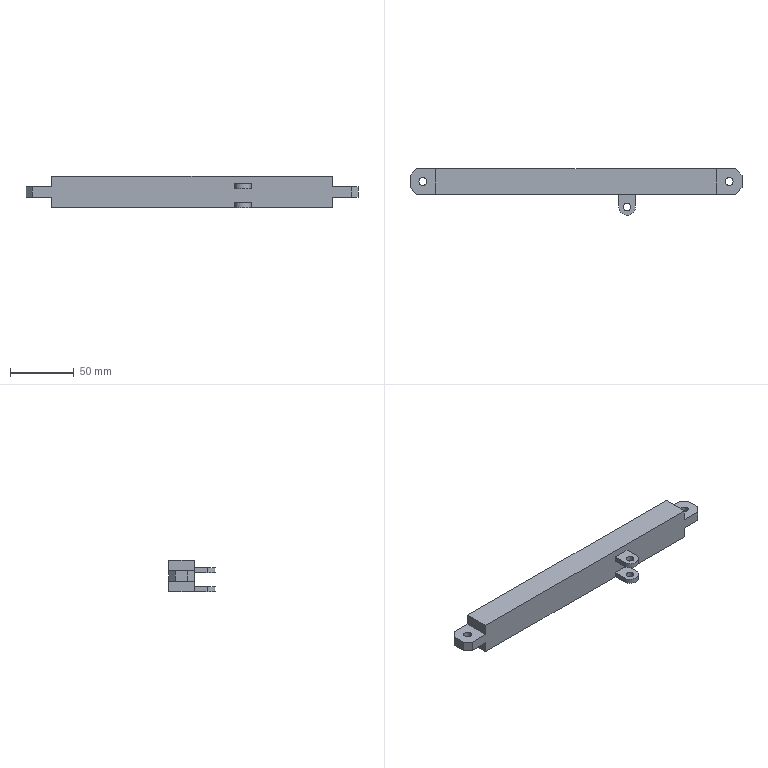Part | SolidWorks | features ICE 3, Chamfer 1, Extrusion 1, LPattern 1, MirrorPattern 1 | 1 solid | 35 faces | box 260 x 36.5 x 25 mm | volume 116892 mm3 | plane 25 | cylinder 10 | commonest cylinder face diameters 6 x8 13 x2
STEP:
#1=CARTESIAN_POINT('',(43.,-20.,6.5));
#2=VERTEX_POINT('',#1);
#3=CARTESIAN_POINT('',(37.,-20.,6.5));
#4=VERTEX_POINT('',#3);
#5=CARTESIAN_POINT('',(40.,-20.,6.5));
#6=DIRECTION('',(0.,0.,-1.));
#7=DIRECTION('',(-1.,0.,0.));
#8=AXIS2_PLACEMENT_3D('',#5,#6,#7);
#9=CIRCLE('',#8,3.);
#10=EDGE_CURVE('',#2,#4,#9,.T.);
#11=ORIENTED_EDGE('',*,*,#10,.F.);
#12=CARTESIAN_POINT('',(43.,-20.,2.5));
#13=VERTEX_POINT('',#12);
#14=CARTESIAN_POINT('',(43.,-20.,6.5));
#15=DIRECTION('',(0.,0.,-1.));
#16=VECTOR('',#15,1000.);
#17=LINE('',#14,#16);
#18=EDGE_CURVE('',#2,#13,#17,.T.);
#19=ORIENTED_EDGE('',*,*,#18,.T.);
#20=CARTESIAN_POINT('',(37.,-20.,2.5));
#21=VERTEX_POINT('',#20);
#22=CARTESIAN_POINT('',(40.,-20.,2.5));
#23=DIRECTION('',(0.,0.,-1.));
#24=DIRECTION('',(-1.,0.,0.));
#25=AXIS2_PLACEMENT_3D('',#22,#23,#24);
#26=CIRCLE('',#25,3.);
#27=EDGE_CURVE('',#13,#21,#26,.T.);
#28=ORIENTED_EDGE('',*,*,#27,.T.);
#29=CARTESIAN_POINT('',(37.,-20.,6.5));
#30=DIRECTION('',(0.,0.,-1.));
#31=VECTOR('',#30,1000.);
#32=LINE('',#29,#31);
#33=EDGE_CURVE('',#4,#21,#32,.T.);
#34=ORIENTED_EDGE('',*,*,#33,.F.);
#35=EDGE_LOOP('',(#11,#19,#28,#34));
#36=FACE_OUTER_BOUND('',#35,.T.);
#37=CARTESIAN_POINT('',(40.,-20.,6.5));
#38=DIRECTION('',(0.,0.,-1.));
#39=DIRECTION('',(-1.,0.,0.));
#40=AXIS2_PLACEMENT_3D('',#37,#38,#39);
#41=CYLINDRICAL_SURFACE('',#40,3.);
#42=ADVANCED_FACE('',(#36),#41,.F.);
#43=CARTESIAN_POINT('',(43.,-20.,-8.5));
#44=VERTEX_POINT('',#43);
#45=CARTESIAN_POINT('',(37.,-20.,-8.5));
#46=VERTEX_POINT('',#45);
#47=CARTESIAN_POINT('',(40.,-20.,-8.5));
#48=DIRECTION('',(0.,0.,-1.));
#49=DIRECTION('',(-1.,0.,0.));
#50=AXIS2_PLACEMENT_3D('',#47,#48,#49);
#51=CIRCLE('',#50,3.);
#52=EDGE_CURVE('',#44,#46,#51,.T.);
#53=ORIENTED_EDGE('',*,*,#52,.F.);
#54=CARTESIAN_POINT('',(43.,-20.,-12.5));
#55=VERTEX_POINT('',#54);
#56=CARTESIAN_POINT('',(43.,-20.,-8.5));
#57=DIRECTION('',(0.,0.,-1.));
#58=VECTOR('',#57,1000.);
#59=LINE('',#56,#58);
#60=EDGE_CURVE('',#44,#55,#59,.T.);
#61=ORIENTED_EDGE('',*,*,#60,.T.);
#62=CARTESIAN_POINT('',(37.,-20.,-12.5));
#63=VERTEX_POINT('',#62);
#64=CARTESIAN_POINT('',(40.,-20.,-12.5));
#65=DIRECTION('',(0.,0.,-1.));
#66=DIRECTION('',(-1.,0.,0.));
#67=AXIS2_PLACEMENT_3D('',#64,#65,#66);
#68=CIRCLE('',#67,3.);
#69=EDGE_CURVE('',#55,#63,#68,.T.);
#70=ORIENTED_EDGE('',*,*,#69,.T.);
#71=CARTESIAN_POINT('',(37.,-20.,-8.5));
#72=DIRECTION('',(0.,0.,-1.));
#73=VECTOR('',#72,1000.);
#74=LINE('',#71,#73);
#75=EDGE_CURVE('',#46,#63,#74,.T.);
#76=ORIENTED_EDGE('',*,*,#75,.F.);
#77=EDGE_LOOP('',(#53,#61,#70,#76));
#78=FACE_OUTER_BOUND('',#77,.T.);
#79=CARTESIAN_POINT('',(40.,-20.,-8.5));
#80=DIRECTION('',(0.,0.,-1.));
#81=DIRECTION('',(-1.,0.,0.));
#82=AXIS2_PLACEMENT_3D('',#79,#80,#81);
#83=CYLINDRICAL_SURFACE('',#82,3.);
#84=ADVANCED_FACE('',(#78),#83,.F.);
#85=CARTESIAN_POINT('',(-117.,0.,-4.));
#86=VERTEX_POINT('',#85);
#87=CARTESIAN_POINT('',(-123.,0.,-4.));
#88=VERTEX_POINT('',#87);
#89=CARTESIAN_POINT('',(-120.,0.,-4.));
#90=DIRECTION('',(0.,0.,-1.));
#91=DIRECTION('',(1.,0.,0.));
#92=AXIS2_PLACEMENT_3D('',#89,#90,#91);
#93=CIRCLE('',#92,3.);
#94=EDGE_CURVE('',#86,#88,#93,.T.);
#95=ORIENTED_EDGE('',*,*,#94,.T.);
#96=CARTESIAN_POINT('',(-123.,0.,4.));
#97=VERTEX_POINT('',#96);
#98=CARTESIAN_POINT('',(-123.,0.,-12.5));
#99=DIRECTION('',(0.,0.,1.));
#100=VECTOR('',#99,1000.);
#101=LINE('',#98,#100);
#102=EDGE_CURVE('',#88,#97,#101,.T.);
#103=ORIENTED_EDGE('',*,*,#102,.T.);
#104=CARTESIAN_POINT('',(-117.,0.,4.));
#105=VERTEX_POINT('',#104);
#106=CARTESIAN_POINT('',(-120.,0.,4.));
#107=DIRECTION('',(0.,0.,1.));
#108=DIRECTION('',(-1.,0.,0.));
#109=AXIS2_PLACEMENT_3D('',#106,#107,#108);
#110=CIRCLE('',#109,3.);
#111=EDGE_CURVE('',#97,#105,#110,.T.);
#112=ORIENTED_EDGE('',*,*,#111,.T.);
#113=CARTESIAN_POINT('',(-117.,0.,-12.5));
#114=DIRECTION('',(0.,0.,1.));
#115=VECTOR('',#114,1000.);
#116=LINE('',#113,#115);
#117=EDGE_CURVE('',#86,#105,#116,.T.);
#118=ORIENTED_EDGE('',*,*,#117,.F.);
#119=EDGE_LOOP('',(#95,#103,#112,#118));
#120=FACE_OUTER_BOUND('',#119,.T.);
#121=CARTESIAN_POINT('',(-120.,0.,-12.5));
#122=DIRECTION('',(0.,0.,1.));
#123=DIRECTION('',(1.,0.,0.));
#124=AXIS2_PLACEMENT_3D('',#121,#122,#123);
#125=CYLINDRICAL_SURFACE('',#124,3.);
#126=ADVANCED_FACE('',(#120),#125,.F.);
#127=CARTESIAN_POINT('',(117.,0.,-4.));
#128=VERTEX_POINT('',#127);
#129=CARTESIAN_POINT('',(123.,0.,-4.));
#130=VERTEX_POINT('',#129);
#131=CARTESIAN_POINT('',(120.,0.,-4.));
#132=DIRECTION('',(0.,0.,1.));
#133=DIRECTION('',(-1.,0.,0.));
#134=AXIS2_PLACEMENT_3D('',#131,#132,#133);
#135=CIRCLE('',#134,3.);
#136=EDGE_CURVE('',#128,#130,#135,.T.);
#137=ORIENTED_EDGE('',*,*,#136,.F.);
#138=CARTESIAN_POINT('',(117.,0.,4.));
#139=VERTEX_POINT('',#138);
#140=CARTESIAN_POINT('',(117.,0.,-12.5));
#141=DIRECTION('',(0.,0.,1.));
#142=VECTOR('',#141,1000.);
#143=LINE('',#140,#142);
#144=EDGE_CURVE('',#128,#139,#143,.T.);
#145=ORIENTED_EDGE('',*,*,#144,.T.);
#146=CARTESIAN_POINT('',(123.,0.,4.));
#147=VERTEX_POINT('',#146);
#148=CARTESIAN_POINT('',(120.,0.,4.));
#149=DIRECTION('',(0.,0.,-1.));
#150=DIRECTION('',(1.,0.,0.));
#151=AXIS2_PLACEMENT_3D('',#148,#149,#150);
#152=CIRCLE('',#151,3.);
#153=EDGE_CURVE('',#147,#139,#152,.T.);
#154=ORIENTED_EDGE('',*,*,#153,.F.);
#155=CARTESIAN_POINT('',(123.,0.,-12.5));
#156=DIRECTION('',(0.,0.,1.));
#157=VECTOR('',#156,1000.);
#158=LINE('',#155,#157);
#159=EDGE_CURVE('',#130,#147,#158,.T.);
#160=ORIENTED_EDGE('',*,*,#159,.F.);
#161=EDGE_LOOP('',(#137,#145,#154,#160));
#162=FACE_OUTER_BOUND('',#161,.T.);
#163=CARTESIAN_POINT('',(120.,0.,-12.5));
#164=DIRECTION('',(0.,0.,1.));
#165=DIRECTION('',(1.,0.,0.));
#166=AXIS2_PLACEMENT_3D('',#163,#164,#165);
#167=CYLINDRICAL_SURFACE('',#166,3.);
#168=ADVANCED_FACE('',(#162),#167,.F.);
#169=CARTESIAN_POINT('',(33.5,-10.,-8.5));
#170=VERTEX_POINT('',#169);
#171=CARTESIAN_POINT('',(33.5,-10.,-12.5));
#172=VERTEX_POINT('',#171);
#173=CARTESIAN_POINT('',(33.5,-10.,-8.5));
#174=DIRECTION('',(0.,0.,-1.));
#175=VECTOR('',#174,1000.);
#176=LINE('',#173,#175);
#177=EDGE_CURVE('',#170,#172,#176,.T.);
#178=ORIENTED_EDGE('',*,*,#177,.F.);
#179=CARTESIAN_POINT('',(46.5,-10.,-8.5));
#180=VERTEX_POINT('',#179);
#181=CARTESIAN_POINT('',(46.5,-10.,-8.5));
#182=DIRECTION('',(1.,0.,0.));
#183=VECTOR('',#182,1000.);
#184=LINE('',#181,#183);
#185=EDGE_CURVE('',#170,#180,#184,.T.);
#186=ORIENTED_EDGE('',*,*,#185,.T.);
#187=CARTESIAN_POINT('',(46.5,-10.,-12.5));
#188=VERTEX_POINT('',#187);
#189=CARTESIAN_POINT('',(46.5,-10.,-8.5));
#190=DIRECTION('',(0.,0.,-1.));
#191=VECTOR('',#190,1000.);
#192=LINE('',#189,#191);
#193=EDGE_CURVE('',#180,#188,#192,.T.);
#194=ORIENTED_EDGE('',*,*,#193,.T.);
#195=CARTESIAN_POINT('',(110.,-10.,-12.5));
#196=VERTEX_POINT('',#195);
#197=CARTESIAN_POINT('',(-130.,-10.,-12.5));
#198=DIRECTION('',(1.,0.,0.));
#199=VECTOR('',#198,1000.);
#200=LINE('',#197,#199);
#201=EDGE_CURVE('',#188,#196,#200,.T.);
#202=ORIENTED_EDGE('',*,*,#201,.T.);
#203=CARTESIAN_POINT('',(110.,-10.,-4.));
#204=VERTEX_POINT('',#203);
#205=CARTESIAN_POINT('',(110.,-10.,-4.));
#206=DIRECTION('',(0.,0.,-1.));
#207=VECTOR('',#206,1000.);
#208=LINE('',#205,#207);
#209=EDGE_CURVE('',#204,#196,#208,.T.);
#210=ORIENTED_EDGE('',*,*,#209,.F.);
#211=CARTESIAN_POINT('',(125.,-10.,-4.));
#212=VERTEX_POINT('',#211);
#213=CARTESIAN_POINT('',(130.,-10.,-4.));
#214=DIRECTION('',(1.,0.,0.));
#215=VECTOR('',#214,1000.);
#216=LINE('',#213,#215);
#217=EDGE_CURVE('',#204,#212,#216,.T.);
#218=ORIENTED_EDGE('',*,*,#217,.T.);
#219=CARTESIAN_POINT('',(125.,-10.,4.));
#220=VERTEX_POINT('',#219);
#221=CARTESIAN_POINT('',(125.,-10.,12.5));
#222=DIRECTION('',(0.,0.,1.));
#223=VECTOR('',#222,1000.);
#224=LINE('',#221,#223);
#225=EDGE_CURVE('',#212,#220,#224,.T.);
#226=ORIENTED_EDGE('',*,*,#225,.T.);
#227=CARTESIAN_POINT('',(110.,-10.,4.));
#228=VERTEX_POINT('',#227);
#229=CARTESIAN_POINT('',(130.,-10.,4.));
#230=DIRECTION('',(1.,0.,0.));
#231=VECTOR('',#230,1000.);
#232=LINE('',#229,#231);
#233=EDGE_CURVE('',#228,#220,#232,.T.);
#234=ORIENTED_EDGE('',*,*,#233,.F.);
#235=CARTESIAN_POINT('',(110.,-10.,12.5));
#236=VERTEX_POINT('',#235);
#237=CARTESIAN_POINT('',(110.,-10.,4.));
#238=DIRECTION('',(0.,0.,1.));
#239=VECTOR('',#238,1000.);
#240=LINE('',#237,#239);
#241=EDGE_CURVE('',#228,#236,#240,.T.);
#242=ORIENTED_EDGE('',*,*,#241,.T.);
#243=CARTESIAN_POINT('',(-110.,-10.,12.5));
#244=VERTEX_POINT('',#243);
#245=CARTESIAN_POINT('',(-130.,-10.,12.5));
#246=DIRECTION('',(1.,0.,0.));
#247=VECTOR('',#246,1000.);
#248=LINE('',#245,#247);
#249=EDGE_CURVE('',#244,#236,#248,.T.);
#250=ORIENTED_EDGE('',*,*,#249,.F.);
#251=CARTESIAN_POINT('',(-110.,-10.,4.));
#252=VERTEX_POINT('',#251);
#253=CARTESIAN_POINT('',(-110.,-10.,4.));
#254=DIRECTION('',(0.,0.,1.));
#255=VECTOR('',#254,1000.);
#256=LINE('',#253,#255);
#257=EDGE_CURVE('',#252,#244,#256,.T.);
#258=ORIENTED_EDGE('',*,*,#257,.F.);
#259=CARTESIAN_POINT('',(-125.,-10.,4.));
#260=VERTEX_POINT('',#259);
#261=CARTESIAN_POINT('',(-130.,-10.,4.));
#262=DIRECTION('',(1.,0.,0.));
#263=VECTOR('',#262,1000.);
#264=LINE('',#261,#263);
#265=EDGE_CURVE('',#260,#252,#264,.T.);
#266=ORIENTED_EDGE('',*,*,#265,.F.);
#267=CARTESIAN_POINT('',(-125.,-10.,-4.));
#268=VERTEX_POINT('',#267);
#269=CARTESIAN_POINT('',(-125.,-10.,12.5));
#270=DIRECTION('',(0.,0.,-1.));
#271=VECTOR('',#270,1000.);
#272=LINE('',#269,#271);
#273=EDGE_CURVE('',#260,#268,#272,.T.);
#274=ORIENTED_EDGE('',*,*,#273,.T.);
#275=CARTESIAN_POINT('',(-110.,-10.,-4.));
#276=VERTEX_POINT('',#275);
#277=CARTESIAN_POINT('',(-130.,-10.,-4.));
#278=DIRECTION('',(1.,0.,0.));
#279=VECTOR('',#278,1000.);
#280=LINE('',#277,#279);
#281=EDGE_CURVE('',#268,#276,#280,.T.);
#282=ORIENTED_EDGE('',*,*,#281,.T.);
#283=CARTESIAN_POINT('',(-110.,-10.,-12.5));
#284=VERTEX_POINT('',#283);
#285=CARTESIAN_POINT('',(-110.,-10.,-4.));
#286=DIRECTION('',(0.,0.,-1.));
#287=VECTOR('',#286,1000.);
#288=LINE('',#285,#287);
#289=EDGE_CURVE('',#276,#284,#288,.T.);
#290=ORIENTED_EDGE('',*,*,#289,.T.);
#291=CARTESIAN_POINT('',(-130.,-10.,-12.5));
#292=DIRECTION('',(1.,0.,0.));
#293=VECTOR('',#292,1000.);
#294=LINE('',#291,#293);
#295=EDGE_CURVE('',#284,#172,#294,.T.);
#296=ORIENTED_EDGE('',*,*,#295,.T.);
#297=EDGE_LOOP('',(#178,#186,#194,#202,#210,#218,#226,#234,#242,#250,#258,#266,#274,#282,#290,#296));
#298=FACE_OUTER_BOUND('',#297,.T.);
#299=CARTESIAN_POINT('',(33.5,-10.,6.5));
#300=VERTEX_POINT('',#299);
#301=CARTESIAN_POINT('',(46.5,-10.,6.5));
#302=VERTEX_POINT('',#301);
#303=CARTESIAN_POINT('',(46.5,-10.,6.5));
#304=DIRECTION('',(1.,0.,0.));
#305=VECTOR('',#304,1000.);
#306=LINE('',#303,#305);
#307=EDGE_CURVE('',#300,#302,#306,.T.);
#308=ORIENTED_EDGE('',*,*,#307,.T.);
#309=CARTESIAN_POINT('',(46.5,-10.,2.5));
#310=VERTEX_POINT('',#309);
#311=CARTESIAN_POINT('',(46.5,-10.,6.5));
#312=DIRECTION('',(0.,0.,-1.));
#313=VECTOR('',#312,1000.);
#314=LINE('',#311,#313);
#315=EDGE_CURVE('',#302,#310,#314,.T.);
#316=ORIENTED_EDGE('',*,*,#315,.T.);
#317=CARTESIAN_POINT('',(33.5,-10.,2.5));
#318=VERTEX_POINT('',#317);
#319=CARTESIAN_POINT('',(46.5,-10.,2.5));
#320=DIRECTION('',(1.,0.,0.));
#321=VECTOR('',#320,1000.);
#322=LINE('',#319,#321);
#323=EDGE_CURVE('',#318,#310,#322,.T.);
#324=ORIENTED_EDGE('',*,*,#323,.F.);
#325=CARTESIAN_POINT('',(33.5,-10.,6.5));
#326=DIRECTION('',(0.,0.,-1.));
#327=VECTOR('',#326,1000.);
#328=LINE('',#325,#327);
#329=EDGE_CURVE('',#300,#318,#328,.T.);
#330=ORIENTED_EDGE('',*,*,#329,.F.);
#331=EDGE_LOOP('',(#308,#316,#324,#330));
#332=FACE_BOUND('',#331,.T.);
#333=CARTESIAN_POINT('',(-130.,-10.,12.5));
#334=DIRECTION('',(0.,1.,0.));
#335=DIRECTION('',(0.,0.,1.));
#336=AXIS2_PLACEMENT_3D('',#333,#334,#335);
#337=PLANE('',#336);
#338=ADVANCED_FACE('',(#298,#332),#337,.F.);
#339=CARTESIAN_POINT('',(130.,-5.,-4.));
#340=VERTEX_POINT('',#339);
#341=CARTESIAN_POINT('',(130.,5.,-4.));
#342=VERTEX_POINT('',#341);
#343=CARTESIAN_POINT('',(130.,10.,-4.));
#344=DIRECTION('',(0.,1.,0.));
#345=VECTOR('',#344,1000.);
#346=LINE('',#343,#345);
#347=EDGE_CURVE('',#340,#342,#346,.T.);
#348=ORIENTED_EDGE('',*,*,#347,.T.);
#349=CARTESIAN_POINT('',(130.,5.,4.));
#350=VERTEX_POINT('',#349);
#351=CARTESIAN_POINT('',(130.,5.,12.5));
#352=DIRECTION('',(0.,0.,1.));
#353=VECTOR('',#352,1000.);
#354=LINE('',#351,#353);
#355=EDGE_CURVE('',#342,#350,#354,.T.);
#356=ORIENTED_EDGE('',*,*,#355,.T.);
#357=CARTESIAN_POINT('',(130.,-5.,4.));
#358=VERTEX_POINT('',#357);
#359=CARTESIAN_POINT('',(130.,10.,4.));
#360=DIRECTION('',(0.,1.,0.));
#361=VECTOR('',#360,1000.);
#362=LINE('',#359,#361);
#363=EDGE_CURVE('',#358,#350,#362,.T.);
#364=ORIENTED_EDGE('',*,*,#363,.F.);
#365=CARTESIAN_POINT('',(130.,-5.,12.5));
#366=DIRECTION('',(0.,0.,-1.));
#367=VECTOR('',#366,1000.);
#368=LINE('',#365,#367);
#369=EDGE_CURVE('',#358,#340,#368,.T.);
#370=ORIENTED_EDGE('',*,*,#369,.T.);
#371=EDGE_LOOP('',(#348,#356,#364,#370));
#372=FACE_OUTER_BOUND('',#371,.T.);
#373=CARTESIAN_POINT('',(130.,10.,12.5));
#374=DIRECTION('',(-1.,0.,0.));
#375=DIRECTION('',(0.,0.,1.));
#376=AXIS2_PLACEMENT_3D('',#373,#374,#375);
#377=PLANE('',#376);
#378=ADVANCED_FACE('',(#372),#377,.F.);
#379=ORIENTED_EDGE('',*,*,#144,.F.);
#380=CARTESIAN_POINT('',(120.,0.,-4.));
#381=DIRECTION('',(0.,0.,1.));
#382=DIRECTION('',(-1.,0.,0.));
#383=AXIS2_PLACEMENT_3D('',#380,#381,#382);
#384=CIRCLE('',#383,3.);
#385=EDGE_CURVE('',#130,#128,#384,.T.);
#386=ORIENTED_EDGE('',*,*,#385,.F.);
#387=ORIENTED_EDGE('',*,*,#159,.T.);
#388=CARTESIAN_POINT('',(120.,0.,4.));
#389=DIRECTION('',(0.,0.,-1.));
#390=DIRECTION('',(1.,0.,0.));
#391=AXIS2_PLACEMENT_3D('',#388,#389,#390);
#392=CIRCLE('',#391,3.);
#393=EDGE_CURVE('',#139,#147,#392,.T.);
#394=ORIENTED_EDGE('',*,*,#393,.F.);
#395=EDGE_LOOP('',(#379,#386,#387,#394));
#396=FACE_OUTER_BOUND('',#395,.T.);
#397=CARTESIAN_POINT('',(120.,0.,-12.5));
#398=DIRECTION('',(0.,0.,1.));
#399=DIRECTION('',(1.,0.,0.));
#400=AXIS2_PLACEMENT_3D('',#397,#398,#399);
#401=CYLINDRICAL_SURFACE('',#400,3.);
#402=ADVANCED_FACE('',(#396),#401,.F.);
#403=CARTESIAN_POINT('',(125.,10.,4.));
#404=VERTEX_POINT('',#403);
#405=CARTESIAN_POINT('',(110.,10.,4.));
#406=VERTEX_POINT('',#405);
#407=CARTESIAN_POINT('',(130.,10.,4.));
#408=DIRECTION('',(-1.,0.,0.));
#409=VECTOR('',#408,1000.);
#410=LINE('',#407,#409);
#411=EDGE_CURVE('',#404,#406,#410,.T.);
#412=ORIENTED_EDGE('',*,*,#411,.F.);
#413=CARTESIAN_POINT('',(125.,10.,-4.));
#414=VERTEX_POINT('',#413);
#415=CARTESIAN_POINT('',(125.,10.,12.5));
#416=DIRECTION('',(0.,0.,-1.));
#417=VECTOR('',#416,1000.);
#418=LINE('',#415,#417);
#419=EDGE_CURVE('',#404,#414,#418,.T.);
#420=ORIENTED_EDGE('',*,*,#419,.T.);
#421=CARTESIAN_POINT('',(110.,10.,-4.));
#422=VERTEX_POINT('',#421);
#423=CARTESIAN_POINT('',(130.,10.,-4.));
#424=DIRECTION('',(-1.,0.,0.));
#425=VECTOR('',#424,1000.);
#426=LINE('',#423,#425);
#427=EDGE_CURVE('',#414,#422,#426,.T.);
#428=ORIENTED_EDGE('',*,*,#427,.T.);
#429=CARTESIAN_POINT('',(110.,10.,-12.5));
#430=VERTEX_POINT('',#429);
#431=CARTESIAN_POINT('',(110.,10.,-4.));
#432=DIRECTION('',(0.,0.,-1.));
#433=VECTOR('',#432,1000.);
#434=LINE('',#431,#433);
#435=EDGE_CURVE('',#422,#430,#434,.T.);
#436=ORIENTED_EDGE('',*,*,#435,.T.);
#437=CARTESIAN_POINT('',(-110.,10.,-12.5));
#438=VERTEX_POINT('',#437);
#439=CARTESIAN_POINT('',(-130.,10.,-12.5));
#440=DIRECTION('',(-1.,0.,0.));
#441=VECTOR('',#440,1000.);
#442=LINE('',#439,#441);
#443=EDGE_CURVE('',#430,#438,#442,.T.);
#444=ORIENTED_EDGE('',*,*,#443,.T.);
#445=CARTESIAN_POINT('',(-110.,10.,-4.));
#446=VERTEX_POINT('',#445);
#447=CARTESIAN_POINT('',(-110.,10.,-4.));
#448=DIRECTION('',(0.,0.,-1.));
#449=VECTOR('',#448,1000.);
#450=LINE('',#447,#449);
#451=EDGE_CURVE('',#446,#438,#450,.T.);
#452=ORIENTED_EDGE('',*,*,#451,.F.);
#453=CARTESIAN_POINT('',(-125.,10.,-4.));
#454=VERTEX_POINT('',#453);
#455=CARTESIAN_POINT('',(-130.,10.,-4.));
#456=DIRECTION('',(-1.,0.,0.));
#457=VECTOR('',#456,1000.);
#458=LINE('',#455,#457);
#459=EDGE_CURVE('',#446,#454,#458,.T.);
#460=ORIENTED_EDGE('',*,*,#459,.T.);
#461=CARTESIAN_POINT('',(-125.,10.,4.));
#462=VERTEX_POINT('',#461);
#463=CARTESIAN_POINT('',(-125.,10.,12.5));
#464=DIRECTION('',(0.,0.,1.));
#465=VECTOR('',#464,1000.);
#466=LINE('',#463,#465);
#467=EDGE_CURVE('',#454,#462,#466,.T.);
#468=ORIENTED_EDGE('',*,*,#467,.T.);
#469=CARTESIAN_POINT('',(-110.,10.,4.));
#470=VERTEX_POINT('',#469);
#471=CARTESIAN_POINT('',(-130.,10.,4.));
#472=DIRECTION('',(-1.,0.,0.));
#473=VECTOR('',#472,1000.);
#474=LINE('',#471,#473);
#475=EDGE_CURVE('',#470,#462,#474,.T.);
#476=ORIENTED_EDGE('',*,*,#475,.F.);
#477=CARTESIAN_POINT('',(-110.,10.,12.5));
#478=VERTEX_POINT('',#477);
#479=CARTESIAN_POINT('',(-110.,10.,4.));
#480=DIRECTION('',(0.,0.,1.));
#481=VECTOR('',#480,1000.);
#482=LINE('',#479,#481);
#483=EDGE_CURVE('',#470,#478,#482,.T.);
#484=ORIENTED_EDGE('',*,*,#483,.T.);
#485=CARTESIAN_POINT('',(110.,10.,12.5));
#486=VERTEX_POINT('',#485);
#487=CARTESIAN_POINT('',(-130.,10.,12.5));
#488=DIRECTION('',(-1.,0.,0.));
#489=VECTOR('',#488,1000.);
#490=LINE('',#487,#489);
#491=EDGE_CURVE('',#486,#478,#490,.T.);
#492=ORIENTED_EDGE('',*,*,#491,.F.);
#493=CARTESIAN_POINT('',(110.,10.,4.));
#494=DIRECTION('',(0.,0.,1.));
#495=VECTOR('',#494,1000.);
#496=LINE('',#493,#495);
#497=EDGE_CURVE('',#406,#486,#496,.T.);
#498=ORIENTED_EDGE('',*,*,#497,.F.);
#499=EDGE_LOOP('',(#412,#420,#428,#436,#444,#452,#460,#468,#476,#484,#492,#498));
#500=FACE_OUTER_BOUND('',#499,.T.);
#501=CARTESIAN_POINT('',(-130.,10.,12.5));
#502=DIRECTION('',(0.,-1.,0.));
#503=DIRECTION('',(0.,0.,-1.));
#504=AXIS2_PLACEMENT_3D('',#501,#502,#503);
#505=PLANE('',#504);
#506=ADVANCED_FACE('',(#500),#505,.F.);
#507=CARTESIAN_POINT('',(-110.,10.,-12.5));
#508=DIRECTION('',(0.,1.,0.));
#509=VECTOR('',#508,1000.);
#510=LINE('',#507,#509);
#511=EDGE_CURVE('',#284,#438,#510,.T.);
#512=ORIENTED_EDGE('',*,*,#511,.T.);
#513=ORIENTED_EDGE('',*,*,#443,.F.);
#514=CARTESIAN_POINT('',(110.,10.,-12.5));
#515=DIRECTION('',(0.,-1.,0.));
#516=VECTOR('',#515,1000.);
#517=LINE('',#514,#516);
#518=EDGE_CURVE('',#430,#196,#517,.T.);
#519=ORIENTED_EDGE('',*,*,#518,.T.);
#520=ORIENTED_EDGE('',*,*,#201,.F.);
#521=CARTESIAN_POINT('',(46.5,-20.,-12.5));
#522=VERTEX_POINT('',#521);
#523=CARTESIAN_POINT('',(46.5,-20.,-12.5));
#524=DIRECTION('',(0.,-1.,0.));
#525=VECTOR('',#524,1000.);
#526=LINE('',#523,#525);
#527=EDGE_CURVE('',#188,#522,#526,.T.);
#528=ORIENTED_EDGE('',*,*,#527,.T.);
#529=CARTESIAN_POINT('',(33.5,-20.,-12.5));
#530=VERTEX_POINT('',#529);
#531=CARTESIAN_POINT('',(40.,-20.,-12.5));
#532=DIRECTION('',(0.,0.,-1.));
#533=DIRECTION('',(-1.,0.,0.));
#534=AXIS2_PLACEMENT_3D('',#531,#532,#533);
#535=CIRCLE('',#534,6.5);
#536=EDGE_CURVE('',#522,#530,#535,.T.);
#537=ORIENTED_EDGE('',*,*,#536,.T.);
#538=CARTESIAN_POINT('',(33.5,-10.,-12.5));
#539=DIRECTION('',(0.,1.,0.));
#540=VECTOR('',#539,1000.);
#541=LINE('',#538,#540);
#542=EDGE_CURVE('',#530,#172,#541,.T.);
#543=ORIENTED_EDGE('',*,*,#542,.T.);
#544=ORIENTED_EDGE('',*,*,#295,.F.);
#545=EDGE_LOOP('',(#512,#513,#519,#520,#528,#537,#543,#544));
#546=FACE_OUTER_BOUND('',#545,.T.);
#547=CARTESIAN_POINT('',(40.,-20.,-12.5));
#548=DIRECTION('',(0.,0.,-1.));
#549=DIRECTION('',(-1.,0.,0.));
#550=AXIS2_PLACEMENT_3D('',#547,#548,#549);
#551=CIRCLE('',#550,3.);
#552=EDGE_CURVE('',#63,#55,#551,.T.);
#553=ORIENTED_EDGE('',*,*,#552,.F.);
#554=ORIENTED_EDGE('',*,*,#69,.F.);
#555=EDGE_LOOP('',(#553,#554));
#556=FACE_BOUND('',#555,.T.);
#557=CARTESIAN_POINT('',(0.,0.,-12.5));
#558=DIRECTION('',(0.,0.,1.));
#559=DIRECTION('',(1.,0.,0.));
#560=AXIS2_PLACEMENT_3D('',#557,#558,#559);
#561=PLANE('',#560);
#562=ADVANCED_FACE('',(#546,#556),#561,.F.);
#563=CARTESIAN_POINT('',(-130.,5.,-4.));
#564=VERTEX_POINT('',#563);
#565=CARTESIAN_POINT('',(-130.,-5.,-4.));
#566=VERTEX_POINT('',#565);
#567=CARTESIAN_POINT('',(-130.,10.,-4.));
#568=DIRECTION('',(0.,-1.,0.));
#569=VECTOR('',#568,1000.);
#570=LINE('',#567,#569);
#571=EDGE_CURVE('',#564,#566,#570,.T.);
#572=ORIENTED_EDGE('',*,*,#571,.T.);
#573=CARTESIAN_POINT('',(-130.,-5.,4.));
#574=VERTEX_POINT('',#573);
#575=CARTESIAN_POINT('',(-130.,-5.,12.5));
#576=DIRECTION('',(0.,0.,1.));
#577=VECTOR('',#576,1000.);
#578=LINE('',#575,#577);
#579=EDGE_CURVE('',#566,#574,#578,.T.);
#580=ORIENTED_EDGE('',*,*,#579,.T.);
#581=CARTESIAN_POINT('',(-130.,5.,4.));
#582=VERTEX_POINT('',#581);
#583=CARTESIAN_POINT('',(-130.,10.,4.));
#584=DIRECTION('',(0.,-1.,0.));
#585=VECTOR('',#584,1000.);
#586=LINE('',#583,#585);
#587=EDGE_CURVE('',#582,#574,#586,.T.);
#588=ORIENTED_EDGE('',*,*,#587,.F.);
#589=CARTESIAN_POINT('',(-130.,5.,12.5));
#590=DIRECTION('',(0.,0.,-1.));
#591=VECTOR('',#590,1000.);
#592=LINE('',#589,#591);
#593=EDGE_CURVE('',#582,#564,#592,.T.);
#594=ORIENTED_EDGE('',*,*,#593,.T.);
#595=EDGE_LOOP('',(#572,#580,#588,#594));
#596=FACE_OUTER_BOUND('',#595,.T.);
#597=CARTESIAN_POINT('',(-130.,10.,12.5));
#598=DIRECTION('',(1.,0.,0.));
#599=DIRECTION('',(0.,0.,-1.));
#600=AXIS2_PLACEMENT_3D('',#597,#598,#599);
#601=PLANE('',#600);
#602=ADVANCED_FACE('',(#596),#601,.F.);
#603=CARTESIAN_POINT('',(-110.,10.,12.5));
#604=DIRECTION('',(0.,1.,0.));
#605=VECTOR('',#604,1000.);
#606=LINE('',#603,#605);
#607=EDGE_CURVE('',#244,#478,#606,.T.);
#608=ORIENTED_EDGE('',*,*,#607,.F.);
#609=ORIENTED_EDGE('',*,*,#249,.T.);
#610=CARTESIAN_POINT('',(110.,10.,12.5));
#611=DIRECTION('',(0.,-1.,0.));
#612=VECTOR('',#611,1000.);
#613=LINE('',#610,#612);
#614=EDGE_CURVE('',#486,#236,#613,.T.);
#615=ORIENTED_EDGE('',*,*,#614,.F.);
#616=ORIENTED_EDGE('',*,*,#491,.T.);
#617=EDGE_LOOP('',(#608,#609,#615,#616));
#618=FACE_OUTER_BOUND('',#617,.T.);
#619=CARTESIAN_POINT('',(0.,0.,12.5));
#620=DIRECTION('',(0.,0.,1.));
#621=DIRECTION('',(1.,0.,0.));
#622=AXIS2_PLACEMENT_3D('',#619,#620,#621);
#623=PLANE('',#622);
#624=ADVANCED_FACE('',(#618),#623,.T.);
#625=ORIENTED_EDGE('',*,*,#102,.F.);
#626=CARTESIAN_POINT('',(-120.,0.,-4.));
#627=DIRECTION('',(0.,0.,-1.));
#628=DIRECTION('',(1.,0.,0.));
#629=AXIS2_PLACEMENT_3D('',#626,#627,#628);
#630=CIRCLE('',#629,3.);
#631=EDGE_CURVE('',#88,#86,#630,.T.);
#632=ORIENTED_EDGE('',*,*,#631,.T.);
#633=ORIENTED_EDGE('',*,*,#117,.T.);
#634=CARTESIAN_POINT('',(-120.,0.,4.));
#635=DIRECTION('',(0.,0.,1.));
#636=DIRECTION('',(-1.,0.,0.));
#637=AXIS2_PLACEMENT_3D('',#634,#635,#636);
#638=CIRCLE('',#637,3.);
#639=EDGE_CURVE('',#105,#97,#638,.T.);
#640=ORIENTED_EDGE('',*,*,#639,.T.);
#641=EDGE_LOOP('',(#625,#632,#633,#640));
#642=FACE_OUTER_BOUND('',#641,.T.);
#643=CARTESIAN_POINT('',(-120.,0.,-12.5));
#644=DIRECTION('',(0.,0.,1.));
#645=DIRECTION('',(1.,0.,0.));
#646=AXIS2_PLACEMENT_3D('',#643,#644,#645);
#647=CYLINDRICAL_SURFACE('',#646,3.);
#648=ADVANCED_FACE('',(#642),#647,.F.);
#649=ORIENTED_EDGE('',*,*,#587,.T.);
#650=CARTESIAN_POINT('',(-125.,-10.,4.));
#651=DIRECTION('',(0.7071,-0.7071,0.));
#652=VECTOR('',#651,1000.);
#653=LINE('',#650,#652);
#654=EDGE_CURVE('',#574,#260,#653,.T.);
#655=ORIENTED_EDGE('',*,*,#654,.T.);
#656=ORIENTED_EDGE('',*,*,#265,.T.);
#657=CARTESIAN_POINT('',(-110.,10.,4.));
#658=DIRECTION('',(0.,1.,0.));
#659=VECTOR('',#658,1000.);
#660=LINE('',#657,#659);
#661=EDGE_CURVE('',#252,#470,#660,.T.);
#662=ORIENTED_EDGE('',*,*,#661,.T.);
#663=ORIENTED_EDGE('',*,*,#475,.T.);
#664=CARTESIAN_POINT('',(-130.,5.,4.));
#665=DIRECTION('',(-0.7071,-0.7071,0.));
#666=VECTOR('',#665,1000.);
#667=LINE('',#664,#666);
#668=EDGE_CURVE('',#462,#582,#667,.T.);
#669=ORIENTED_EDGE('',*,*,#668,.T.);
#670=EDGE_LOOP('',(#649,#655,#656,#662,#663,#669));
#671=FACE_OUTER_BOUND('',#670,.T.);
#672=ORIENTED_EDGE('',*,*,#639,.F.);
#673=ORIENTED_EDGE('',*,*,#111,.F.);
#674=EDGE_LOOP('',(#672,#673));
#675=FACE_BOUND('',#674,.T.);
#676=CARTESIAN_POINT('',(0.,0.,4.));
#677=DIRECTION('',(0.,0.,-1.));
#678=DIRECTION('',(-1.,0.,0.));
#679=AXIS2_PLACEMENT_3D('',#676,#677,#678);
#680=PLANE('',#679);
#681=ADVANCED_FACE('',(#671,#675),#680,.F.);
#682=ORIENTED_EDGE('',*,*,#607,.T.);
#683=ORIENTED_EDGE('',*,*,#483,.F.);
#684=ORIENTED_EDGE('',*,*,#661,.F.);
#685=ORIENTED_EDGE('',*,*,#257,.T.);
#686=EDGE_LOOP('',(#682,#683,#684,#685));
#687=FACE_OUTER_BOUND('',#686,.T.);
#688=CARTESIAN_POINT('',(-110.,10.,4.));
#689=DIRECTION('',(1.,0.,0.));
#690=DIRECTION('',(0.,0.,-1.));
#691=AXIS2_PLACEMENT_3D('',#688,#689,#690);
#692=PLANE('',#691);
#693=ADVANCED_FACE('',(#687),#692,.F.);
#694=ORIENTED_EDGE('',*,*,#363,.T.);
#695=CARTESIAN_POINT('',(67.5,67.5,4.));
#696=DIRECTION('',(-0.7071,0.7071,0.));
#697=VECTOR('',#696,1000.);
#698=LINE('',#695,#697);
#699=EDGE_CURVE('',#350,#404,#698,.T.);
#700=ORIENTED_EDGE('',*,*,#699,.T.);
#701=ORIENTED_EDGE('',*,*,#411,.T.);
#702=CARTESIAN_POINT('',(110.,10.,4.));
#703=DIRECTION('',(0.,-1.,0.));
#704=VECTOR('',#703,1000.);
#705=LINE('',#702,#704);
#706=EDGE_CURVE('',#406,#228,#705,.T.);
#707=ORIENTED_EDGE('',*,*,#706,.T.);
#708=ORIENTED_EDGE('',*,*,#233,.T.);
#709=CARTESIAN_POINT('',(67.5,-67.5,4.));
#710=DIRECTION('',(0.7071,0.7071,0.));
#711=VECTOR('',#710,1000.);
#712=LINE('',#709,#711);
#713=EDGE_CURVE('',#220,#358,#712,.T.);
#714=ORIENTED_EDGE('',*,*,#713,.T.);
#715=EDGE_LOOP('',(#694,#700,#701,#707,#708,#714));
#716=FACE_OUTER_BOUND('',#715,.T.);
#717=ORIENTED_EDGE('',*,*,#153,.T.);
#718=ORIENTED_EDGE('',*,*,#393,.T.);
#719=EDGE_LOOP('',(#717,#718));
#720=FACE_BOUND('',#719,.T.);
#721=CARTESIAN_POINT('',(0.,0.,4.));
#722=DIRECTION('',(0.,0.,1.));
#723=DIRECTION('',(1.,0.,0.));
#724=AXIS2_PLACEMENT_3D('',#721,#722,#723);
#725=PLANE('',#724);
#726=ADVANCED_FACE('',(#716,#720),#725,.T.);
#727=ORIENTED_EDGE('',*,*,#614,.T.);
#728=ORIENTED_EDGE('',*,*,#241,.F.);
#729=ORIENTED_EDGE('',*,*,#706,.F.);
#730=ORIENTED_EDGE('',*,*,#497,.T.);
#731=EDGE_LOOP('',(#727,#728,#729,#730));
#732=FACE_OUTER_BOUND('',#731,.T.);
#733=CARTESIAN_POINT('',(110.,10.,4.));
#734=DIRECTION('',(-1.,0.,0.));
#735=DIRECTION('',(0.,0.,1.));
#736=AXIS2_PLACEMENT_3D('',#733,#734,#735);
#737=PLANE('',#736);
#738=ADVANCED_FACE('',(#732),#737,.F.);
#739=ORIENTED_EDGE('',*,*,#281,.F.);
#740=CARTESIAN_POINT('',(-125.,-10.,-4.));
#741=DIRECTION('',(-0.7071,0.7071,0.));
#742=VECTOR('',#741,1000.);
#743=LINE('',#740,#742);
#744=EDGE_CURVE('',#268,#566,#743,.T.);
#745=ORIENTED_EDGE('',*,*,#744,.T.);
#746=ORIENTED_EDGE('',*,*,#571,.F.);
#747=CARTESIAN_POINT('',(-130.,5.,-4.));
#748=DIRECTION('',(0.7071,0.7071,0.));
#749=VECTOR('',#748,1000.);
#750=LINE('',#747,#749);
#751=EDGE_CURVE('',#564,#454,#750,.T.);
#752=ORIENTED_EDGE('',*,*,#751,.T.);
#753=ORIENTED_EDGE('',*,*,#459,.F.);
#754=CARTESIAN_POINT('',(-110.,10.,-4.));
#755=DIRECTION('',(0.,1.,0.));
#756=VECTOR('',#755,1000.);
#757=LINE('',#754,#756);
#758=EDGE_CURVE('',#276,#446,#757,.T.);
#759=ORIENTED_EDGE('',*,*,#758,.F.);
#760=EDGE_LOOP('',(#739,#745,#746,#752,#753,#759));
#761=FACE_OUTER_BOUND('',#760,.T.);
#762=ORIENTED_EDGE('',*,*,#94,.F.);
#763=ORIENTED_EDGE('',*,*,#631,.F.);
#764=EDGE_LOOP('',(#762,#763));
#765=FACE_BOUND('',#764,.T.);
#766=CARTESIAN_POINT('',(0.,0.,-4.));
#767=DIRECTION('',(0.,0.,1.));
#768=DIRECTION('',(-1.,0.,0.));
#769=AXIS2_PLACEMENT_3D('',#766,#767,#768);
#770=PLANE('',#769);
#771=ADVANCED_FACE('',(#761,#765),#770,.F.);
#772=ORIENTED_EDGE('',*,*,#511,.F.);
#773=ORIENTED_EDGE('',*,*,#289,.F.);
#774=ORIENTED_EDGE('',*,*,#758,.T.);
#775=ORIENTED_EDGE('',*,*,#451,.T.);
#776=EDGE_LOOP('',(#772,#773,#774,#775));
#777=FACE_OUTER_BOUND('',#776,.T.);
#778=CARTESIAN_POINT('',(-110.,10.,-4.));
#779=DIRECTION('',(-1.,0.,0.));
#780=DIRECTION('',(0.,0.,1.));
#781=AXIS2_PLACEMENT_3D('',#778,#779,#780);
#782=PLANE('',#781);
#783=ADVANCED_FACE('',(#777),#782,.T.);
#784=ORIENTED_EDGE('',*,*,#427,.F.);
#785=CARTESIAN_POINT('',(67.5,67.5,-4.));
#786=DIRECTION('',(0.7071,-0.7071,0.));
#787=VECTOR('',#786,1000.);
#788=LINE('',#785,#787);
#789=EDGE_CURVE('',#414,#342,#788,.T.);
#790=ORIENTED_EDGE('',*,*,#789,.T.);
#791=ORIENTED_EDGE('',*,*,#347,.F.);
#792=CARTESIAN_POINT('',(67.5,-67.5,-4.));
#793=DIRECTION('',(-0.7071,-0.7071,0.));
#794=VECTOR('',#793,1000.);
#795=LINE('',#792,#794);
#796=EDGE_CURVE('',#340,#212,#795,.T.);
#797=ORIENTED_EDGE('',*,*,#796,.T.);
#798=ORIENTED_EDGE('',*,*,#217,.F.);
#799=CARTESIAN_POINT('',(110.,10.,-4.));
#800=DIRECTION('',(0.,-1.,0.));
#801=VECTOR('',#800,1000.);
#802=LINE('',#799,#801);
#803=EDGE_CURVE('',#422,#204,#802,.T.);
#804=ORIENTED_EDGE('',*,*,#803,.F.);
#805=EDGE_LOOP('',(#784,#790,#791,#797,#798,#804));
#806=FACE_OUTER_BOUND('',#805,.T.);
#807=ORIENTED_EDGE('',*,*,#385,.T.);
#808=ORIENTED_EDGE('',*,*,#136,.T.);
#809=EDGE_LOOP('',(#807,#808));
#810=FACE_BOUND('',#809,.T.);
#811=CARTESIAN_POINT('',(0.,0.,-4.));
#812=DIRECTION('',(0.,0.,-1.));
#813=DIRECTION('',(1.,0.,0.));
#814=AXIS2_PLACEMENT_3D('',#811,#812,#813);
#815=PLANE('',#814);
#816=ADVANCED_FACE('',(#806,#810),#815,.T.);
#817=ORIENTED_EDGE('',*,*,#518,.F.);
#818=ORIENTED_EDGE('',*,*,#435,.F.);
#819=ORIENTED_EDGE('',*,*,#803,.T.);
#820=ORIENTED_EDGE('',*,*,#209,.T.);
#821=EDGE_LOOP('',(#817,#818,#819,#820));
#822=FACE_OUTER_BOUND('',#821,.T.);
#823=CARTESIAN_POINT('',(110.,10.,-4.));
#824=DIRECTION('',(1.,0.,0.));
#825=DIRECTION('',(0.,0.,-1.));
#826=AXIS2_PLACEMENT_3D('',#823,#824,#825);
#827=PLANE('',#826);
#828=ADVANCED_FACE('',(#822),#827,.T.);
#829=ORIENTED_EDGE('',*,*,#699,.F.);
#830=ORIENTED_EDGE('',*,*,#355,.F.);
#831=ORIENTED_EDGE('',*,*,#789,.F.);
#832=ORIENTED_EDGE('',*,*,#419,.F.);
#833=EDGE_LOOP('',(#829,#830,#831,#832));
#834=FACE_OUTER_BOUND('',#833,.T.);
#835=CARTESIAN_POINT('',(125.,10.,12.5));
#836=DIRECTION('',(-0.7071,-0.7071,0.));
#837=DIRECTION('',(0.,0.,-1.));
#838=AXIS2_PLACEMENT_3D('',#835,#836,#837);
#839=PLANE('',#838);
#840=ADVANCED_FACE('',(#834),#839,.F.);
#841=ORIENTED_EDGE('',*,*,#713,.F.);
#842=ORIENTED_EDGE('',*,*,#225,.F.);
#843=ORIENTED_EDGE('',*,*,#796,.F.);
#844=ORIENTED_EDGE('',*,*,#369,.F.);
#845=EDGE_LOOP('',(#841,#842,#843,#844));
#846=FACE_OUTER_BOUND('',#845,.T.);
#847=CARTESIAN_POINT('',(130.,-5.,12.5));
#848=DIRECTION('',(-0.7071,0.7071,0.));
#849=DIRECTION('',(0.,0.,-1.));
#850=AXIS2_PLACEMENT_3D('',#847,#848,#849);
#851=PLANE('',#850);
#852=ADVANCED_FACE('',(#846),#851,.F.);
#853=ORIENTED_EDGE('',*,*,#654,.F.);
#854=ORIENTED_EDGE('',*,*,#579,.F.);
#855=ORIENTED_EDGE('',*,*,#744,.F.);
#856=ORIENTED_EDGE('',*,*,#273,.F.);
#857=EDGE_LOOP('',(#853,#854,#855,#856));
#858=FACE_OUTER_BOUND('',#857,.T.);
#859=CARTESIAN_POINT('',(-125.,-10.,12.5));
#860=DIRECTION('',(0.7071,0.7071,0.));
#861=DIRECTION('',(0.,0.,-1.));
#862=AXIS2_PLACEMENT_3D('',#859,#860,#861);
#863=PLANE('',#862);
#864=ADVANCED_FACE('',(#858),#863,.F.);
#865=ORIENTED_EDGE('',*,*,#668,.F.);
#866=ORIENTED_EDGE('',*,*,#467,.F.);
#867=ORIENTED_EDGE('',*,*,#751,.F.);
#868=ORIENTED_EDGE('',*,*,#593,.F.);
#869=EDGE_LOOP('',(#865,#866,#867,#868));
#870=FACE_OUTER_BOUND('',#869,.T.);
#871=CARTESIAN_POINT('',(-130.,5.,12.5));
#872=DIRECTION('',(0.7071,-0.7071,0.));
#873=DIRECTION('',(0.,0.,-1.));
#874=AXIS2_PLACEMENT_3D('',#871,#872,#873);
#875=PLANE('',#874);
#876=ADVANCED_FACE('',(#870),#875,.F.);
#877=ORIENTED_EDGE('',*,*,#542,.F.);
#878=CARTESIAN_POINT('',(33.5,-20.,-8.5));
#879=VERTEX_POINT('',#878);
#880=CARTESIAN_POINT('',(33.5,-20.,-8.5));
#881=DIRECTION('',(0.,0.,-1.));
#882=VECTOR('',#881,1000.);
#883=LINE('',#880,#882);
#884=EDGE_CURVE('',#879,#530,#883,.T.);
#885=ORIENTED_EDGE('',*,*,#884,.F.);
#886=CARTESIAN_POINT('',(33.5,-10.,-8.5));
#887=DIRECTION('',(0.,1.,0.));
#888=VECTOR('',#887,1000.);
#889=LINE('',#886,#888);
#890=EDGE_CURVE('',#879,#170,#889,.T.);
#891=ORIENTED_EDGE('',*,*,#890,.T.);
#892=ORIENTED_EDGE('',*,*,#177,.T.);
#893=EDGE_LOOP('',(#877,#885,#891,#892));
#894=FACE_OUTER_BOUND('',#893,.T.);
#895=CARTESIAN_POINT('',(33.5,-10.,-8.5));
#896=DIRECTION('',(-1.,0.,0.));
#897=DIRECTION('',(0.,-1.,0.));
#898=AXIS2_PLACEMENT_3D('',#895,#896,#897);
#899=PLANE('',#898);
#900=ADVANCED_FACE('',(#894),#899,.T.);
#901=ORIENTED_EDGE('',*,*,#536,.F.);
#902=CARTESIAN_POINT('',(46.5,-20.,-8.5));
#903=VERTEX_POINT('',#902);
#904=CARTESIAN_POINT('',(46.5,-20.,-8.5));
#905=DIRECTION('',(0.,0.,-1.));
#906=VECTOR('',#905,1000.);
#907=LINE('',#904,#906);
#908=EDGE_CURVE('',#903,#522,#907,.T.);
#909=ORIENTED_EDGE('',*,*,#908,.F.);
#910=CARTESIAN_POINT('',(40.,-20.,-8.5));
#911=DIRECTION('',(0.,0.,-1.));
#912=DIRECTION('',(-1.,0.,0.));
#913=AXIS2_PLACEMENT_3D('',#910,#911,#912);
#914=CIRCLE('',#913,6.5);
#915=EDGE_CURVE('',#903,#879,#914,.T.);
#916=ORIENTED_EDGE('',*,*,#915,.T.);
#917=ORIENTED_EDGE('',*,*,#884,.T.);
#918=EDGE_LOOP('',(#901,#909,#916,#917));
#919=FACE_OUTER_BOUND('',#918,.T.);
#920=CARTESIAN_POINT('',(40.,-20.,-8.5));
#921=DIRECTION('',(0.,0.,-1.));
#922=DIRECTION('',(-1.,0.,0.));
#923=AXIS2_PLACEMENT_3D('',#920,#921,#922);
#924=CYLINDRICAL_SURFACE('',#923,6.5);
#925=ADVANCED_FACE('',(#919),#924,.T.);
#926=ORIENTED_EDGE('',*,*,#527,.F.);
#927=ORIENTED_EDGE('',*,*,#193,.F.);
#928=CARTESIAN_POINT('',(46.5,-20.,-8.5));
#929=DIRECTION('',(0.,-1.,0.));
#930=VECTOR('',#929,1000.);
#931=LINE('',#928,#930);
#932=EDGE_CURVE('',#180,#903,#931,.T.);
#933=ORIENTED_EDGE('',*,*,#932,.T.);
#934=ORIENTED_EDGE('',*,*,#908,.T.);
#935=EDGE_LOOP('',(#926,#927,#933,#934));
#936=FACE_OUTER_BOUND('',#935,.T.);
#937=CARTESIAN_POINT('',(46.5,-20.,-8.5));
#938=DIRECTION('',(1.,0.,0.));
#939=DIRECTION('',(0.,0.,-1.));
#940=AXIS2_PLACEMENT_3D('',#937,#938,#939);
#941=PLANE('',#940);
#942=ADVANCED_FACE('',(#936),#941,.T.);
#943=CARTESIAN_POINT('',(40.,-20.,-8.5));
#944=DIRECTION('',(0.,0.,-1.));
#945=DIRECTION('',(-1.,0.,0.));
#946=AXIS2_PLACEMENT_3D('',#943,#944,#945);
#947=CIRCLE('',#946,3.);
#948=EDGE_CURVE('',#46,#44,#947,.T.);
#949=ORIENTED_EDGE('',*,*,#948,.T.);
#950=ORIENTED_EDGE('',*,*,#52,.T.);
#951=EDGE_LOOP('',(#949,#950));
#952=FACE_BOUND('',#951,.T.);
#953=ORIENTED_EDGE('',*,*,#890,.F.);
#954=ORIENTED_EDGE('',*,*,#915,.F.);
#955=ORIENTED_EDGE('',*,*,#932,.F.);
#956=ORIENTED_EDGE('',*,*,#185,.F.);
#957=EDGE_LOOP('',(#953,#954,#955,#956));
#958=FACE_OUTER_BOUND('',#957,.T.);
#959=CARTESIAN_POINT('',(40.,-20.,-8.5));
#960=DIRECTION('',(0.,0.,-1.));
#961=DIRECTION('',(-1.,0.,0.));
#962=AXIS2_PLACEMENT_3D('',#959,#960,#961);
#963=PLANE('',#962);
#964=ADVANCED_FACE('',(#952,#958),#963,.F.);
#965=ORIENTED_EDGE('',*,*,#60,.F.);
#966=ORIENTED_EDGE('',*,*,#948,.F.);
#967=ORIENTED_EDGE('',*,*,#75,.T.);
#968=ORIENTED_EDGE('',*,*,#552,.T.);
#969=EDGE_LOOP('',(#965,#966,#967,#968));
#970=FACE_OUTER_BOUND('',#969,.T.);
#971=CARTESIAN_POINT('',(40.,-20.,-8.5));
#972=DIRECTION('',(0.,0.,-1.));
#973=DIRECTION('',(-1.,0.,0.));
#974=AXIS2_PLACEMENT_3D('',#971,#972,#973);
#975=CYLINDRICAL_SURFACE('',#974,3.);
#976=ADVANCED_FACE('',(#970),#975,.F.);
#977=CARTESIAN_POINT('',(33.5,-20.,2.5));
#978=VERTEX_POINT('',#977);
#979=CARTESIAN_POINT('',(33.5,-10.,2.5));
#980=DIRECTION('',(0.,1.,0.));
#981=VECTOR('',#980,1000.);
#982=LINE('',#979,#981);
#983=EDGE_CURVE('',#978,#318,#982,.T.);
#984=ORIENTED_EDGE('',*,*,#983,.F.);
#985=CARTESIAN_POINT('',(33.5,-20.,6.5));
#986=VERTEX_POINT('',#985);
#987=CARTESIAN_POINT('',(33.5,-20.,6.5));
#988=DIRECTION('',(0.,0.,-1.));
#989=VECTOR('',#988,1000.);
#990=LINE('',#987,#989);
#991=EDGE_CURVE('',#986,#978,#990,.T.);
#992=ORIENTED_EDGE('',*,*,#991,.F.);
#993=CARTESIAN_POINT('',(33.5,-10.,6.5));
#994=DIRECTION('',(0.,1.,0.));
#995=VECTOR('',#994,1000.);
#996=LINE('',#993,#995);
#997=EDGE_CURVE('',#986,#300,#996,.T.);
#998=ORIENTED_EDGE('',*,*,#997,.T.);
#999=ORIENTED_EDGE('',*,*,#329,.T.);
#1000=EDGE_LOOP('',(#984,#992,#998,#999));
#1001=FACE_OUTER_BOUND('',#1000,.T.);
#1002=CARTESIAN_POINT('',(33.5,-10.,6.5));
#1003=DIRECTION('',(-1.,0.,0.));
#1004=DIRECTION('',(0.,-1.,0.));
#1005=AXIS2_PLACEMENT_3D('',#1002,#1003,#1004);
#1006=PLANE('',#1005);
#1007=ADVANCED_FACE('',(#1001),#1006,.T.);
#1008=CARTESIAN_POINT('',(46.5,-20.,2.5));
#1009=VERTEX_POINT('',#1008);
#1010=CARTESIAN_POINT('',(40.,-20.,2.5));
#1011=DIRECTION('',(0.,0.,-1.));
#1012=DIRECTION('',(-1.,0.,0.));
#1013=AXIS2_PLACEMENT_3D('',#1010,#1011,#1012);
#1014=CIRCLE('',#1013,6.5);
#1015=EDGE_CURVE('',#1009,#978,#1014,.T.);
#1016=ORIENTED_EDGE('',*,*,#1015,.F.);
#1017=CARTESIAN_POINT('',(46.5,-20.,6.5));
#1018=VERTEX_POINT('',#1017);
#1019=CARTESIAN_POINT('',(46.5,-20.,6.5));
#1020=DIRECTION('',(0.,0.,-1.));
#1021=VECTOR('',#1020,1000.);
#1022=LINE('',#1019,#1021);
#1023=EDGE_CURVE('',#1018,#1009,#1022,.T.);
#1024=ORIENTED_EDGE('',*,*,#1023,.F.);
#1025=CARTESIAN_POINT('',(40.,-20.,6.5));
#1026=DIRECTION('',(0.,0.,-1.));
#1027=DIRECTION('',(-1.,0.,0.));
#1028=AXIS2_PLACEMENT_3D('',#1025,#1026,#1027);
#1029=CIRCLE('',#1028,6.5);
#1030=EDGE_CURVE('',#1018,#986,#1029,.T.);
#1031=ORIENTED_EDGE('',*,*,#1030,.T.);
#1032=ORIENTED_EDGE('',*,*,#991,.T.);
#1033=EDGE_LOOP('',(#1016,#1024,#1031,#1032));
#1034=FACE_OUTER_BOUND('',#1033,.T.);
#1035=CARTESIAN_POINT('',(40.,-20.,6.5));
#1036=DIRECTION('',(0.,0.,-1.));
#1037=DIRECTION('',(-1.,0.,0.));
#1038=AXIS2_PLACEMENT_3D('',#1035,#1036,#1037);
#1039=CYLINDRICAL_SURFACE('',#1038,6.5);
#1040=ADVANCED_FACE('',(#1034),#1039,.T.);
#1041=CARTESIAN_POINT('',(46.5,-20.,2.5));
#1042=DIRECTION('',(0.,-1.,0.));
#1043=VECTOR('',#1042,1000.);
#1044=LINE('',#1041,#1043);
#1045=EDGE_CURVE('',#310,#1009,#1044,.T.);
#1046=ORIENTED_EDGE('',*,*,#1045,.F.);
#1047=ORIENTED_EDGE('',*,*,#315,.F.);
#1048=CARTESIAN_POINT('',(46.5,-20.,6.5));
#1049=DIRECTION('',(0.,-1.,0.));
#1050=VECTOR('',#1049,1000.);
#1051=LINE('',#1048,#1050);
#1052=EDGE_CURVE('',#302,#1018,#1051,.T.);
#1053=ORIENTED_EDGE('',*,*,#1052,.T.);
#1054=ORIENTED_EDGE('',*,*,#1023,.T.);
#1055=EDGE_LOOP('',(#1046,#1047,#1053,#1054));
#1056=FACE_OUTER_BOUND('',#1055,.T.);
#1057=CARTESIAN_POINT('',(46.5,-20.,6.5));
#1058=DIRECTION('',(1.,0.,0.));
#1059=DIRECTION('',(0.,0.,-1.));
#1060=AXIS2_PLACEMENT_3D('',#1057,#1058,#1059);
#1061=PLANE('',#1060);
#1062=ADVANCED_FACE('',(#1056),#1061,.T.);
#1063=CARTESIAN_POINT('',(40.,-20.,6.5));
#1064=DIRECTION('',(0.,0.,-1.));
#1065=DIRECTION('',(-1.,0.,0.));
#1066=AXIS2_PLACEMENT_3D('',#1063,#1064,#1065);
#1067=CIRCLE('',#1066,3.);
#1068=EDGE_CURVE('',#4,#2,#1067,.T.);
#1069=ORIENTED_EDGE('',*,*,#1068,.T.);
#1070=ORIENTED_EDGE('',*,*,#10,.T.);
#1071=EDGE_LOOP('',(#1069,#1070));
#1072=FACE_BOUND('',#1071,.T.);
#1073=ORIENTED_EDGE('',*,*,#997,.F.);
#1074=ORIENTED_EDGE('',*,*,#1030,.F.);
#1075=ORIENTED_EDGE('',*,*,#1052,.F.);
#1076=ORIENTED_EDGE('',*,*,#307,.F.);
#1077=EDGE_LOOP('',(#1073,#1074,#1075,#1076));
#1078=FACE_OUTER_BOUND('',#1077,.T.);
#1079=CARTESIAN_POINT('',(40.,-20.,6.5));
#1080=DIRECTION('',(0.,0.,-1.));
#1081=DIRECTION('',(-1.,0.,0.));
#1082=AXIS2_PLACEMENT_3D('',#1079,#1080,#1081);
#1083=PLANE('',#1082);
#1084=ADVANCED_FACE('',(#1072,#1078),#1083,.F.);
#1085=CARTESIAN_POINT('',(40.,-20.,2.5));
#1086=DIRECTION('',(0.,0.,-1.));
#1087=DIRECTION('',(-1.,0.,0.));
#1088=AXIS2_PLACEMENT_3D('',#1085,#1086,#1087);
#1089=CIRCLE('',#1088,3.);
#1090=EDGE_CURVE('',#21,#13,#1089,.T.);
#1091=ORIENTED_EDGE('',*,*,#1090,.F.);
#1092=ORIENTED_EDGE('',*,*,#27,.F.);
#1093=EDGE_LOOP('',(#1091,#1092));
#1094=FACE_BOUND('',#1093,.T.);
#1095=ORIENTED_EDGE('',*,*,#983,.T.);
#1096=ORIENTED_EDGE('',*,*,#323,.T.);
#1097=ORIENTED_EDGE('',*,*,#1045,.T.);
#1098=ORIENTED_EDGE('',*,*,#1015,.T.);
#1099=EDGE_LOOP('',(#1095,#1096,#1097,#1098));
#1100=FACE_OUTER_BOUND('',#1099,.T.);
#1101=CARTESIAN_POINT('',(40.,-20.,2.5));
#1102=DIRECTION('',(0.,0.,-1.));
#1103=DIRECTION('',(-1.,0.,0.));
#1104=AXIS2_PLACEMENT_3D('',#1101,#1102,#1103);
#1105=PLANE('',#1104);
#1106=ADVANCED_FACE('',(#1094,#1100),#1105,.T.);
#1107=ORIENTED_EDGE('',*,*,#18,.F.);
#1108=ORIENTED_EDGE('',*,*,#1068,.F.);
#1109=ORIENTED_EDGE('',*,*,#33,.T.);
#1110=ORIENTED_EDGE('',*,*,#1090,.T.);
#1111=EDGE_LOOP('',(#1107,#1108,#1109,#1110));
#1112=FACE_OUTER_BOUND('',#1111,.T.);
#1113=CARTESIAN_POINT('',(40.,-20.,6.5));
#1114=DIRECTION('',(0.,0.,-1.));
#1115=DIRECTION('',(-1.,0.,0.));
#1116=AXIS2_PLACEMENT_3D('',#1113,#1114,#1115);
#1117=CYLINDRICAL_SURFACE('',#1116,3.);
#1118=ADVANCED_FACE('',(#1112),#1117,.F.);
#1119=CLOSED_SHELL('',(#42,#84,#126,#168,#338,#378,#402,#506,#562,#602,#624,#648,#681,#693,#726,#738,#771,#783,#816,#828,#840,#852,#864,#876,#900,#925,#942,#964,#976,#1007,#1040,#1062,#1084,#1106,#1118));
#1120=MANIFOLD_SOLID_BREP('',#1119);
#1121=CARTESIAN_POINT('',(0.,0.,0.));
#1122=DIRECTION('',(0.,0.,1.));
#1123=DIRECTION('',(1.,0.,0.));
#1124=AXIS2_PLACEMENT_3D('',#1121,#1122,#1123);
#1125=(LENGTH_UNIT()NAMED_UNIT(*)SI_UNIT(.MILLI.,.METRE.));
#1126=UNCERTAINTY_MEASURE_WITH_UNIT(LENGTH_MEASURE(0.00001),#1125,'','');
#1127=(NAMED_UNIT(*)PLANE_ANGLE_UNIT()SI_UNIT($,.RADIAN.));
#1128=(NAMED_UNIT(*)SI_UNIT($,.STERADIAN.)SOLID_ANGLE_UNIT());
#1129=(GEOMETRIC_REPRESENTATION_CONTEXT(3)GLOBAL_UNCERTAINTY_ASSIGNED_CONTEXT((#1126))GLOBAL_UNIT_ASSIGNED_CONTEXT((#1125,#1127,#1128))REPRESENTATION_CONTEXT('',''));
#1130=ADVANCED_BREP_SHAPE_REPRESENTATION('',(#1120,#1124),#1129);